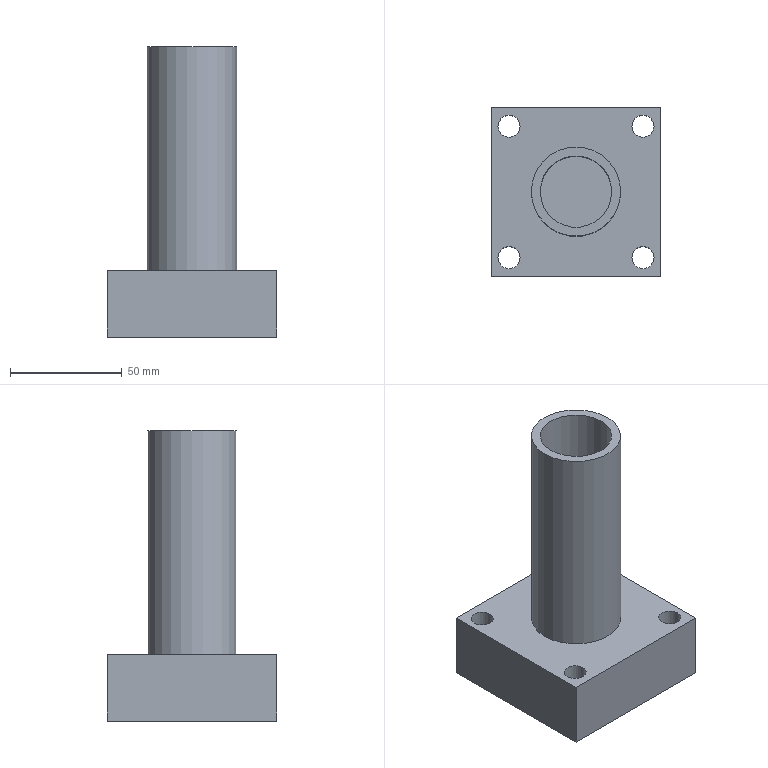Part | NX | features solid 2 | 1 solid | 16 faces | box 76 x 76 x 130 mm | volume 193450 mm3 | plane 9 | cylinder 7 | commonest cylinder face diameters 9.874 x4 18 x1 32 x1 40 x1
STEP:
#1=CARTESIAN_POINT('',(-34.937,-184.406,-280.));
#2=VERTEX_POINT('',#1);
#3=CARTESIAN_POINT('',(-30.,-184.406,-280.));
#4=DIRECTION('',(0.,0.,-1.));
#5=DIRECTION('',(-1.,0.,0.));
#6=AXIS2_PLACEMENT_3D('',#3,#4,#5);
#7=CIRCLE('',#6,4.937);
#8=EDGE_CURVE('',#2,#2,#7,.T.);
#9=ORIENTED_EDGE('',*,*,#8,.T.);
#10=EDGE_LOOP('',(#9));
#11=FACE_BOUND('',#10,.T.);
#12=CARTESIAN_POINT('',(34.937,-184.406,-280.));
#13=VERTEX_POINT('',#12);
#14=CARTESIAN_POINT('',(30.,-184.406,-280.));
#15=DIRECTION('',(0.,0.,1.));
#16=DIRECTION('',(1.,0.,0.));
#17=AXIS2_PLACEMENT_3D('',#14,#15,#16);
#18=CIRCLE('',#17,4.937);
#19=EDGE_CURVE('',#13,#13,#18,.T.);
#20=ORIENTED_EDGE('',*,*,#19,.F.);
#21=EDGE_LOOP('',(#20));
#22=FACE_BOUND('',#21,.T.);
#23=CARTESIAN_POINT('',(38.,-117.,-280.));
#24=VERTEX_POINT('',#23);
#25=CARTESIAN_POINT('',(38.,-193.,-280.));
#26=VERTEX_POINT('',#25);
#27=CARTESIAN_POINT('',(38.,-155.,-280.));
#28=DIRECTION('',(0.,-1.,0.));
#29=VECTOR('',#28,1000.);
#30=LINE('',#27,#29);
#31=EDGE_CURVE('',#24,#26,#30,.T.);
#32=ORIENTED_EDGE('',*,*,#31,.F.);
#33=CARTESIAN_POINT('',(-38.,-117.,-280.));
#34=VERTEX_POINT('',#33);
#35=CARTESIAN_POINT('',(-38.,-117.,-280.));
#36=DIRECTION('',(1.,0.,0.));
#37=VECTOR('',#36,1000.);
#38=LINE('',#35,#37);
#39=EDGE_CURVE('',#34,#24,#38,.T.);
#40=ORIENTED_EDGE('',*,*,#39,.F.);
#41=CARTESIAN_POINT('',(-38.,-193.,-280.));
#42=VERTEX_POINT('',#41);
#43=CARTESIAN_POINT('',(-38.,-155.,-280.));
#44=DIRECTION('',(0.,1.,0.));
#45=VECTOR('',#44,1000.);
#46=LINE('',#43,#45);
#47=EDGE_CURVE('',#42,#34,#46,.T.);
#48=ORIENTED_EDGE('',*,*,#47,.F.);
#49=CARTESIAN_POINT('',(-38.,-193.,-280.));
#50=DIRECTION('',(1.,0.,0.));
#51=VECTOR('',#50,1000.);
#52=LINE('',#49,#51);
#53=EDGE_CURVE('',#42,#26,#52,.T.);
#54=ORIENTED_EDGE('',*,*,#53,.T.);
#55=EDGE_LOOP('',(#32,#40,#48,#54));
#56=FACE_BOUND('',#55,.T.);
#57=CARTESIAN_POINT('',(-34.937,-125.594,-280.));
#58=VERTEX_POINT('',#57);
#59=CARTESIAN_POINT('',(-30.,-125.594,-280.));
#60=DIRECTION('',(0.,0.,1.));
#61=DIRECTION('',(-1.,0.,0.));
#62=AXIS2_PLACEMENT_3D('',#59,#60,#61);
#63=CIRCLE('',#62,4.937);
#64=EDGE_CURVE('',#58,#58,#63,.T.);
#65=ORIENTED_EDGE('',*,*,#64,.F.);
#66=EDGE_LOOP('',(#65));
#67=FACE_BOUND('',#66,.T.);
#68=CARTESIAN_POINT('',(34.937,-125.594,-280.));
#69=VERTEX_POINT('',#68);
#70=CARTESIAN_POINT('',(30.,-125.594,-280.));
#71=DIRECTION('',(0.,0.,-1.));
#72=DIRECTION('',(1.,0.,0.));
#73=AXIS2_PLACEMENT_3D('',#70,#71,#72);
#74=CIRCLE('',#73,4.937);
#75=EDGE_CURVE('',#69,#69,#74,.T.);
#76=ORIENTED_EDGE('',*,*,#75,.T.);
#77=EDGE_LOOP('',(#76));
#78=FACE_BOUND('',#77,.T.);
#79=CARTESIAN_POINT('',(-20.,-155.,-280.));
#80=VERTEX_POINT('',#79);
#81=CARTESIAN_POINT('',(0.,-155.,-280.));
#82=DIRECTION('',(0.,0.,1.));
#83=DIRECTION('',(-1.,0.,0.));
#84=AXIS2_PLACEMENT_3D('',#81,#82,#83);
#85=CIRCLE('',#84,20.);
#86=EDGE_CURVE('',#80,#80,#85,.F.);
#87=ORIENTED_EDGE('',*,*,#86,.T.);
#88=EDGE_LOOP('',(#87));
#89=FACE_BOUND('',#88,.T.);
#90=CARTESIAN_POINT('',(38.,-117.,-280.));
#91=DIRECTION('',(0.,0.,1.));
#92=DIRECTION('',(-1.,0.,0.));
#93=AXIS2_PLACEMENT_3D('',#90,#91,#92);
#94=PLANE('',#93);
#95=ADVANCED_FACE('',(#11,#22,#56,#67,#78,#89),#94,.T.);
#96=CARTESIAN_POINT('',(6.,-117.,-295.));
#97=VERTEX_POINT('',#96);
#98=CARTESIAN_POINT('',(-3.,-117.,-295.));
#99=DIRECTION('',(0.,-1.,0.));
#100=DIRECTION('',(1.,0.,0.));
#101=AXIS2_PLACEMENT_3D('',#98,#99,#100);
#102=CIRCLE('',#101,9.);
#103=EDGE_CURVE('',#97,#97,#102,.T.);
#104=ORIENTED_EDGE('',*,*,#103,.T.);
#105=EDGE_LOOP('',(#104));
#106=FACE_BOUND('',#105,.T.);
#107=CARTESIAN_POINT('',(-38.,-117.,-310.));
#108=VERTEX_POINT('',#107);
#109=CARTESIAN_POINT('',(38.,-117.,-310.));
#110=VERTEX_POINT('',#109);
#111=CARTESIAN_POINT('',(-38.,-117.,-310.));
#112=DIRECTION('',(1.,0.,0.));
#113=VECTOR('',#112,1000.);
#114=LINE('',#111,#113);
#115=EDGE_CURVE('',#108,#110,#114,.T.);
#116=ORIENTED_EDGE('',*,*,#115,.F.);
#117=CARTESIAN_POINT('',(-38.,-117.,-280.));
#118=DIRECTION('',(0.,0.,-1.));
#119=VECTOR('',#118,1000.);
#120=LINE('',#117,#119);
#121=EDGE_CURVE('',#34,#108,#120,.T.);
#122=ORIENTED_EDGE('',*,*,#121,.F.);
#123=ORIENTED_EDGE('',*,*,#39,.T.);
#124=CARTESIAN_POINT('',(38.,-117.,-280.));
#125=DIRECTION('',(0.,0.,-1.));
#126=VECTOR('',#125,1000.);
#127=LINE('',#124,#126);
#128=EDGE_CURVE('',#24,#110,#127,.T.);
#129=ORIENTED_EDGE('',*,*,#128,.T.);
#130=EDGE_LOOP('',(#116,#122,#123,#129));
#131=FACE_BOUND('',#130,.T.);
#132=CARTESIAN_POINT('',(-38.,-117.,-280.));
#133=DIRECTION('',(0.,1.,0.));
#134=DIRECTION('',(-1.,0.,0.));
#135=AXIS2_PLACEMENT_3D('',#132,#133,#134);
#136=PLANE('',#135);
#137=ADVANCED_FACE('',(#106,#131),#136,.T.);
#138=CARTESIAN_POINT('',(-38.,-193.,-310.));
#139=VERTEX_POINT('',#138);
#140=CARTESIAN_POINT('',(-38.,-155.,-310.));
#141=DIRECTION('',(0.,-1.,0.));
#142=VECTOR('',#141,1000.);
#143=LINE('',#140,#142);
#144=EDGE_CURVE('',#108,#139,#143,.T.);
#145=ORIENTED_EDGE('',*,*,#144,.T.);
#146=CARTESIAN_POINT('',(-38.,-193.,-280.));
#147=DIRECTION('',(0.,0.,-1.));
#148=VECTOR('',#147,1000.);
#149=LINE('',#146,#148);
#150=EDGE_CURVE('',#42,#139,#149,.T.);
#151=ORIENTED_EDGE('',*,*,#150,.F.);
#152=ORIENTED_EDGE('',*,*,#47,.T.);
#153=ORIENTED_EDGE('',*,*,#121,.T.);
#154=EDGE_LOOP('',(#145,#151,#152,#153));
#155=FACE_BOUND('',#154,.T.);
#156=CARTESIAN_POINT('',(-38.,-155.,-280.));
#157=DIRECTION('',(1.,0.,0.));
#158=DIRECTION('',(0.,1.,0.));
#159=AXIS2_PLACEMENT_3D('',#156,#157,#158);
#160=PLANE('',#159);
#161=ADVANCED_FACE('',(#155),#160,.F.);
#162=CARTESIAN_POINT('',(38.,-193.,-310.));
#163=VERTEX_POINT('',#162);
#164=CARTESIAN_POINT('',(38.,-193.,-310.));
#165=DIRECTION('',(-1.,0.,0.));
#166=VECTOR('',#165,1000.);
#167=LINE('',#164,#166);
#168=EDGE_CURVE('',#163,#139,#167,.T.);
#169=ORIENTED_EDGE('',*,*,#168,.F.);
#170=CARTESIAN_POINT('',(38.,-193.,-280.));
#171=DIRECTION('',(0.,0.,-1.));
#172=VECTOR('',#171,1000.);
#173=LINE('',#170,#172);
#174=EDGE_CURVE('',#26,#163,#173,.T.);
#175=ORIENTED_EDGE('',*,*,#174,.F.);
#176=ORIENTED_EDGE('',*,*,#53,.F.);
#177=ORIENTED_EDGE('',*,*,#150,.T.);
#178=EDGE_LOOP('',(#169,#175,#176,#177));
#179=FACE_BOUND('',#178,.T.);
#180=CARTESIAN_POINT('',(38.,-193.,-280.));
#181=DIRECTION('',(0.,-1.,0.));
#182=DIRECTION('',(0.,0.,1.));
#183=AXIS2_PLACEMENT_3D('',#180,#181,#182);
#184=PLANE('',#183);
#185=ADVANCED_FACE('',(#179),#184,.T.);
#186=ORIENTED_EDGE('',*,*,#19,.T.);
#187=EDGE_LOOP('',(#186));
#188=FACE_BOUND('',#187,.T.);
#189=CARTESIAN_POINT('',(34.937,-184.406,-310.));
#190=VERTEX_POINT('',#189);
#191=CARTESIAN_POINT('',(30.,-184.406,-310.));
#192=DIRECTION('',(0.,0.,1.));
#193=DIRECTION('',(1.,0.,0.));
#194=AXIS2_PLACEMENT_3D('',#191,#192,#193);
#195=CIRCLE('',#194,4.937);
#196=EDGE_CURVE('',#190,#190,#195,.T.);
#197=ORIENTED_EDGE('',*,*,#196,.F.);
#198=EDGE_LOOP('',(#197));
#199=FACE_BOUND('',#198,.T.);
#200=CARTESIAN_POINT('',(30.,-184.406,-280.));
#201=DIRECTION('',(0.,0.,-1.));
#202=DIRECTION('',(1.,0.,0.));
#203=AXIS2_PLACEMENT_3D('',#200,#201,#202);
#204=CYLINDRICAL_SURFACE('',#203,4.937);
#205=ADVANCED_FACE('',(#188,#199),#204,.F.);
#206=CARTESIAN_POINT('',(38.,-155.,-310.));
#207=DIRECTION('',(0.,1.,0.));
#208=VECTOR('',#207,1000.);
#209=LINE('',#206,#208);
#210=EDGE_CURVE('',#163,#110,#209,.T.);
#211=ORIENTED_EDGE('',*,*,#210,.T.);
#212=ORIENTED_EDGE('',*,*,#128,.F.);
#213=ORIENTED_EDGE('',*,*,#31,.T.);
#214=ORIENTED_EDGE('',*,*,#174,.T.);
#215=EDGE_LOOP('',(#211,#212,#213,#214));
#216=FACE_BOUND('',#215,.T.);
#217=CARTESIAN_POINT('',(38.,-155.,-280.));
#218=DIRECTION('',(-1.,0.,0.));
#219=DIRECTION('',(0.,-1.,0.));
#220=AXIS2_PLACEMENT_3D('',#217,#218,#219);
#221=PLANE('',#220);
#222=ADVANCED_FACE('',(#216),#221,.F.);
#223=ORIENTED_EDGE('',*,*,#64,.T.);
#224=EDGE_LOOP('',(#223));
#225=FACE_BOUND('',#224,.T.);
#226=CARTESIAN_POINT('',(-34.937,-125.594,-310.));
#227=VERTEX_POINT('',#226);
#228=CARTESIAN_POINT('',(-30.,-125.594,-310.));
#229=DIRECTION('',(0.,0.,1.));
#230=DIRECTION('',(-1.,0.,0.));
#231=AXIS2_PLACEMENT_3D('',#228,#229,#230);
#232=CIRCLE('',#231,4.937);
#233=EDGE_CURVE('',#227,#227,#232,.T.);
#234=ORIENTED_EDGE('',*,*,#233,.F.);
#235=EDGE_LOOP('',(#234));
#236=FACE_BOUND('',#235,.T.);
#237=CARTESIAN_POINT('',(-30.,-125.594,-280.));
#238=DIRECTION('',(0.,0.,-1.));
#239=DIRECTION('',(1.,0.,0.));
#240=AXIS2_PLACEMENT_3D('',#237,#238,#239);
#241=CYLINDRICAL_SURFACE('',#240,4.937);
#242=ADVANCED_FACE('',(#225,#236),#241,.F.);
#243=ORIENTED_EDGE('',*,*,#75,.F.);
#244=EDGE_LOOP('',(#243));
#245=FACE_BOUND('',#244,.T.);
#246=CARTESIAN_POINT('',(34.937,-125.594,-310.));
#247=VERTEX_POINT('',#246);
#248=CARTESIAN_POINT('',(30.,-125.594,-310.));
#249=DIRECTION('',(0.,0.,-1.));
#250=DIRECTION('',(1.,0.,0.));
#251=AXIS2_PLACEMENT_3D('',#248,#249,#250);
#252=CIRCLE('',#251,4.937);
#253=EDGE_CURVE('',#247,#247,#252,.T.);
#254=ORIENTED_EDGE('',*,*,#253,.T.);
#255=EDGE_LOOP('',(#254));
#256=FACE_BOUND('',#255,.T.);
#257=CARTESIAN_POINT('',(30.,-125.594,-280.));
#258=DIRECTION('',(0.,0.,-1.));
#259=DIRECTION('',(1.,0.,0.));
#260=AXIS2_PLACEMENT_3D('',#257,#258,#259);
#261=CYLINDRICAL_SURFACE('',#260,4.937);
#262=ADVANCED_FACE('',(#245,#256),#261,.F.);
#263=ORIENTED_EDGE('',*,*,#8,.F.);
#264=EDGE_LOOP('',(#263));
#265=FACE_BOUND('',#264,.T.);
#266=CARTESIAN_POINT('',(-34.937,-184.406,-310.));
#267=VERTEX_POINT('',#266);
#268=CARTESIAN_POINT('',(-30.,-184.406,-310.));
#269=DIRECTION('',(0.,0.,-1.));
#270=DIRECTION('',(-1.,0.,0.));
#271=AXIS2_PLACEMENT_3D('',#268,#269,#270);
#272=CIRCLE('',#271,4.937);
#273=EDGE_CURVE('',#267,#267,#272,.T.);
#274=ORIENTED_EDGE('',*,*,#273,.T.);
#275=EDGE_LOOP('',(#274));
#276=FACE_BOUND('',#275,.T.);
#277=CARTESIAN_POINT('',(-30.,-184.406,-280.));
#278=DIRECTION('',(0.,0.,-1.));
#279=DIRECTION('',(1.,0.,0.));
#280=AXIS2_PLACEMENT_3D('',#277,#278,#279);
#281=CYLINDRICAL_SURFACE('',#280,4.937);
#282=ADVANCED_FACE('',(#265,#276),#281,.F.);
#283=ORIENTED_EDGE('',*,*,#253,.F.);
#284=EDGE_LOOP('',(#283));
#285=FACE_BOUND('',#284,.T.);
#286=ORIENTED_EDGE('',*,*,#233,.T.);
#287=EDGE_LOOP('',(#286));
#288=FACE_BOUND('',#287,.T.);
#289=ORIENTED_EDGE('',*,*,#115,.T.);
#290=ORIENTED_EDGE('',*,*,#210,.F.);
#291=ORIENTED_EDGE('',*,*,#168,.T.);
#292=ORIENTED_EDGE('',*,*,#144,.F.);
#293=EDGE_LOOP('',(#289,#290,#291,#292));
#294=FACE_BOUND('',#293,.T.);
#295=ORIENTED_EDGE('',*,*,#196,.T.);
#296=EDGE_LOOP('',(#295));
#297=FACE_BOUND('',#296,.T.);
#298=ORIENTED_EDGE('',*,*,#273,.F.);
#299=EDGE_LOOP('',(#298));
#300=FACE_BOUND('',#299,.T.);
#301=CARTESIAN_POINT('',(38.,-117.,-310.));
#302=DIRECTION('',(0.,0.,1.));
#303=DIRECTION('',(-1.,0.,0.));
#304=AXIS2_PLACEMENT_3D('',#301,#302,#303);
#305=PLANE('',#304);
#306=ADVANCED_FACE('',(#285,#288,#294,#297,#300),#305,.F.);
#307=ORIENTED_EDGE('',*,*,#86,.F.);
#308=EDGE_LOOP('',(#307));
#309=FACE_BOUND('',#308,.T.);
#310=CARTESIAN_POINT('',(-20.,-155.,-180.));
#311=VERTEX_POINT('',#310);
#312=CARTESIAN_POINT('',(0.,-155.,-180.));
#313=DIRECTION('',(0.,0.,1.));
#314=DIRECTION('',(-1.,0.,0.));
#315=AXIS2_PLACEMENT_3D('',#312,#313,#314);
#316=CIRCLE('',#315,20.);
#317=EDGE_CURVE('',#311,#311,#316,.T.);
#318=ORIENTED_EDGE('',*,*,#317,.F.);
#319=EDGE_LOOP('',(#318));
#320=FACE_BOUND('',#319,.T.);
#321=CARTESIAN_POINT('',(0.,-155.,-180.));
#322=DIRECTION('',(0.,0.,-1.));
#323=DIRECTION('',(1.,0.,0.));
#324=AXIS2_PLACEMENT_3D('',#321,#322,#323);
#325=CYLINDRICAL_SURFACE('',#324,20.);
#326=ADVANCED_FACE('',(#309,#320),#325,.T.);
#327=CARTESIAN_POINT('',(-16.,-155.,-180.));
#328=VERTEX_POINT('',#327);
#329=CARTESIAN_POINT('',(0.,-155.,-180.));
#330=DIRECTION('',(0.,0.,1.));
#331=DIRECTION('',(-1.,0.,0.));
#332=AXIS2_PLACEMENT_3D('',#329,#330,#331);
#333=CIRCLE('',#332,16.);
#334=EDGE_CURVE('',#328,#328,#333,.T.);
#335=ORIENTED_EDGE('',*,*,#334,.F.);
#336=EDGE_LOOP('',(#335));
#337=FACE_BOUND('',#336,.T.);
#338=ORIENTED_EDGE('',*,*,#317,.T.);
#339=EDGE_LOOP('',(#338));
#340=FACE_BOUND('',#339,.T.);
#341=CARTESIAN_POINT('',(0.,-155.,-180.));
#342=DIRECTION('',(0.,0.,1.));
#343=DIRECTION('',(-1.,0.,0.));
#344=AXIS2_PLACEMENT_3D('',#341,#342,#343);
#345=PLANE('',#344);
#346=ADVANCED_FACE('',(#337,#340),#345,.T.);
#347=ORIENTED_EDGE('',*,*,#334,.T.);
#348=EDGE_LOOP('',(#347));
#349=FACE_BOUND('',#348,.T.);
#350=CARTESIAN_POINT('',(-16.,-155.,-295.));
#351=VERTEX_POINT('',#350);
#352=CARTESIAN_POINT('',(0.,-155.,-295.));
#353=DIRECTION('',(0.,0.,1.));
#354=DIRECTION('',(-1.,0.,0.));
#355=AXIS2_PLACEMENT_3D('',#352,#353,#354);
#356=CIRCLE('',#355,16.);
#357=EDGE_CURVE('',#351,#351,#356,.T.);
#358=ORIENTED_EDGE('',*,*,#357,.F.);
#359=EDGE_LOOP('',(#358));
#360=FACE_BOUND('',#359,.T.);
#361=CARTESIAN_POINT('',(0.,-155.,-295.));
#362=DIRECTION('',(0.,0.,1.));
#363=DIRECTION('',(-1.,0.,0.));
#364=AXIS2_PLACEMENT_3D('',#361,#362,#363);
#365=CYLINDRICAL_SURFACE('',#364,16.);
#366=ADVANCED_FACE('',(#349,#360),#365,.F.);
#367=ORIENTED_EDGE('',*,*,#357,.T.);
#368=EDGE_LOOP('',(#367));
#369=FACE_BOUND('',#368,.T.);
#370=CARTESIAN_POINT('',(0.,-155.,-295.));
#371=DIRECTION('',(0.,0.,1.));
#372=DIRECTION('',(-1.,0.,0.));
#373=AXIS2_PLACEMENT_3D('',#370,#371,#372);
#374=PLANE('',#373);
#375=ADVANCED_FACE('',(#369),#374,.T.);
#376=CARTESIAN_POINT('',(6.,-132.,-295.));
#377=VERTEX_POINT('',#376);
#378=CARTESIAN_POINT('',(-3.,-132.,-295.));
#379=DIRECTION('',(0.,-1.,0.));
#380=DIRECTION('',(1.,0.,0.));
#381=AXIS2_PLACEMENT_3D('',#378,#379,#380);
#382=CIRCLE('',#381,9.);
#383=EDGE_CURVE('',#377,#377,#382,.T.);
#384=ORIENTED_EDGE('',*,*,#383,.F.);
#385=EDGE_LOOP('',(#384));
#386=FACE_BOUND('',#385,.T.);
#387=CARTESIAN_POINT('',(-3.,-132.,-295.));
#388=DIRECTION('',(0.,-1.,0.));
#389=DIRECTION('',(1.,0.,0.));
#390=AXIS2_PLACEMENT_3D('',#387,#388,#389);
#391=PLANE('',#390);
#392=ADVANCED_FACE('',(#386),#391,.F.);
#393=ORIENTED_EDGE('',*,*,#383,.T.);
#394=EDGE_LOOP('',(#393));
#395=FACE_BOUND('',#394,.T.);
#396=ORIENTED_EDGE('',*,*,#103,.F.);
#397=EDGE_LOOP('',(#396));
#398=FACE_BOUND('',#397,.T.);
#399=CARTESIAN_POINT('',(-3.,-117.,-295.));
#400=DIRECTION('',(0.,-1.,0.));
#401=DIRECTION('',(1.,0.,0.));
#402=AXIS2_PLACEMENT_3D('',#399,#400,#401);
#403=CYLINDRICAL_SURFACE('',#402,9.);
#404=ADVANCED_FACE('',(#395,#398),#403,.F.);
#405=CLOSED_SHELL('',(#95,#137,#161,#185,#205,#222,#242,#262,#282,#306,#326,#346,#366,#375,#392,#404));
#406=MANIFOLD_SOLID_BREP('',#405);
#407=(LENGTH_UNIT()NAMED_UNIT(*)SI_UNIT(.MILLI.,.METRE.));
#408=UNCERTAINTY_MEASURE_WITH_UNIT(LENGTH_MEASURE(0.00001),#407,'','');
#409=(NAMED_UNIT(*)PLANE_ANGLE_UNIT()SI_UNIT($,.RADIAN.));
#410=(NAMED_UNIT(*)SI_UNIT($,.STERADIAN.)SOLID_ANGLE_UNIT());
#411=(GEOMETRIC_REPRESENTATION_CONTEXT(3)GLOBAL_UNCERTAINTY_ASSIGNED_CONTEXT((#408))GLOBAL_UNIT_ASSIGNED_CONTEXT((#407,#409,#410))REPRESENTATION_CONTEXT('',''));
#412=ADVANCED_BREP_SHAPE_REPRESENTATION('',(#406),#411);